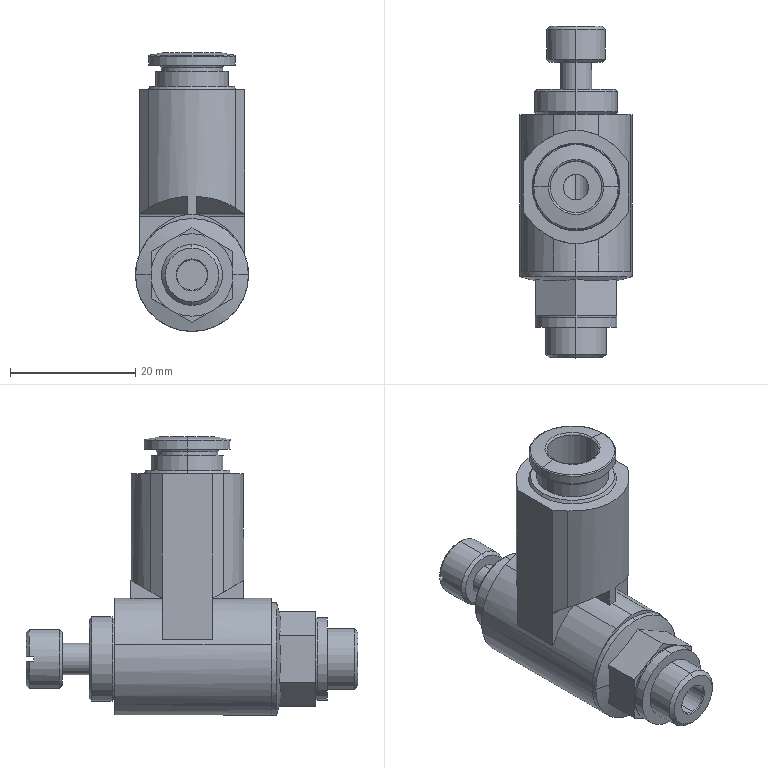Part | SolidWorks | features BaseBody 1 | 1 solid | 120 faces | box 18 x 52.9 x 44.45 mm | volume 12907 mm3 | plane 51 | cylinder 45 | cone 18 | spline 6 | commonest cylinder face diameters 1 x4 4.1 x4 18 x4 20.735 x4 4.864 x2 5 x2